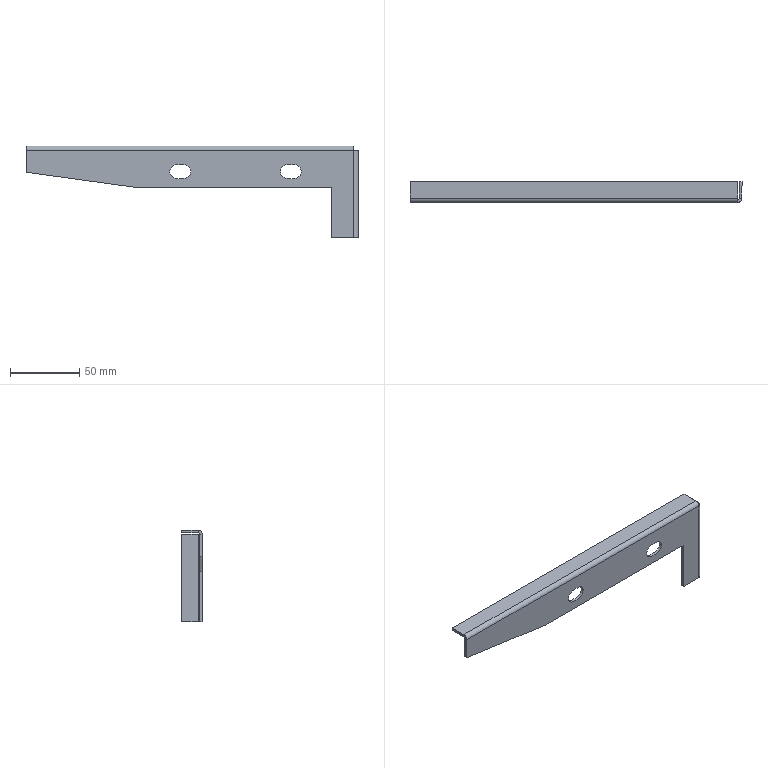Part | 1 solid | 33 faces | box 240 x 15 x 66.5 mm | volume 21672 mm3 | plane 25 | cylinder 8 | commonest cylinder face diameters 10 x4 2 x2 6 x2
STEP:
#1=CARTESIAN_POINT('',(-128.,-2.,43.));
#2=VERTEX_POINT('',#1);
#3=CARTESIAN_POINT('',(-123.,-2.,43.));
#4=VERTEX_POINT('',#3);
#5=CARTESIAN_POINT('',(-128.,-2.,43.));
#6=DIRECTION('',(1.,0.,0.));
#7=VECTOR('',#6,1000.);
#8=LINE('',#5,#7);
#9=EDGE_CURVE('',#2,#4,#8,.T.);
#10=ORIENTED_EDGE('',*,*,#9,.F.);
#11=CARTESIAN_POINT('',(-128.,-2.,53.));
#12=VERTEX_POINT('',#11);
#13=CARTESIAN_POINT('',(-128.,-2.,48.));
#14=DIRECTION('',(0.,-1.,0.));
#15=DIRECTION('',(0.,0.,-1.));
#16=AXIS2_PLACEMENT_3D('',#13,#14,#15);
#17=CIRCLE('',#16,5.);
#18=EDGE_CURVE('',#12,#2,#17,.T.);
#19=ORIENTED_EDGE('',*,*,#18,.F.);
#20=CARTESIAN_POINT('',(-123.,-2.,53.));
#21=VERTEX_POINT('',#20);
#22=CARTESIAN_POINT('',(-128.,-2.,53.));
#23=DIRECTION('',(-1.,0.,0.));
#24=VECTOR('',#23,1000.);
#25=LINE('',#22,#24);
#26=EDGE_CURVE('',#21,#12,#25,.T.);
#27=ORIENTED_EDGE('',*,*,#26,.F.);
#28=CARTESIAN_POINT('',(-123.,-2.,48.));
#29=DIRECTION('',(0.,-1.,0.));
#30=DIRECTION('',(0.,0.,-1.));
#31=AXIS2_PLACEMENT_3D('',#28,#29,#30);
#32=CIRCLE('',#31,5.);
#33=EDGE_CURVE('',#4,#21,#32,.T.);
#34=ORIENTED_EDGE('',*,*,#33,.F.);
#35=EDGE_LOOP('',(#10,#19,#27,#34));
#36=FACE_BOUND('',#35,.T.);
#37=CARTESIAN_POINT('',(-48.,-2.,43.));
#38=VERTEX_POINT('',#37);
#39=CARTESIAN_POINT('',(-43.,-2.,43.));
#40=VERTEX_POINT('',#39);
#41=CARTESIAN_POINT('',(-48.,-2.,43.));
#42=DIRECTION('',(1.,0.,0.));
#43=VECTOR('',#42,1000.);
#44=LINE('',#41,#43);
#45=EDGE_CURVE('',#38,#40,#44,.T.);
#46=ORIENTED_EDGE('',*,*,#45,.F.);
#47=CARTESIAN_POINT('',(-48.,-2.,53.));
#48=VERTEX_POINT('',#47);
#49=CARTESIAN_POINT('',(-48.,-2.,48.));
#50=DIRECTION('',(0.,-1.,0.));
#51=DIRECTION('',(0.,0.,-1.));
#52=AXIS2_PLACEMENT_3D('',#49,#50,#51);
#53=CIRCLE('',#52,5.);
#54=EDGE_CURVE('',#48,#38,#53,.T.);
#55=ORIENTED_EDGE('',*,*,#54,.F.);
#56=CARTESIAN_POINT('',(-43.,-2.,53.));
#57=VERTEX_POINT('',#56);
#58=CARTESIAN_POINT('',(-48.,-2.,53.));
#59=DIRECTION('',(-1.,0.,0.));
#60=VECTOR('',#59,1000.);
#61=LINE('',#58,#60);
#62=EDGE_CURVE('',#57,#48,#61,.T.);
#63=ORIENTED_EDGE('',*,*,#62,.F.);
#64=CARTESIAN_POINT('',(-43.,-2.,48.));
#65=DIRECTION('',(0.,-1.,0.));
#66=DIRECTION('',(0.,0.,-1.));
#67=AXIS2_PLACEMENT_3D('',#64,#65,#66);
#68=CIRCLE('',#67,5.);
#69=EDGE_CURVE('',#40,#57,#68,.T.);
#70=ORIENTED_EDGE('',*,*,#69,.F.);
#71=EDGE_LOOP('',(#46,#55,#63,#70));
#72=FACE_BOUND('',#71,.T.);
#73=CARTESIAN_POINT('',(-237.,-2.,63.5));
#74=VERTEX_POINT('',#73);
#75=CARTESIAN_POINT('',(-237.,-2.,47.5));
#76=VERTEX_POINT('',#75);
#77=CARTESIAN_POINT('',(-237.,-2.,63.5));
#78=DIRECTION('',(0.,0.,-1.));
#79=VECTOR('',#78,1000.);
#80=LINE('',#77,#79);
#81=EDGE_CURVE('',#74,#76,#80,.T.);
#82=ORIENTED_EDGE('',*,*,#81,.T.);
#83=CARTESIAN_POINT('',(-157.,-2.,36.5));
#84=VERTEX_POINT('',#83);
#85=CARTESIAN_POINT('',(-237.,-2.,47.5));
#86=DIRECTION('',(-0.9907,0.,0.1362));
#87=VECTOR('',#86,1000.);
#88=LINE('',#85,#87);
#89=EDGE_CURVE('',#84,#76,#88,.T.);
#90=ORIENTED_EDGE('',*,*,#89,.F.);
#91=CARTESIAN_POINT('',(-16.,-2.,36.5));
#92=VERTEX_POINT('',#91);
#93=CARTESIAN_POINT('',(-237.,-2.,36.5));
#94=DIRECTION('',(-1.,0.,0.));
#95=VECTOR('',#94,1000.);
#96=LINE('',#93,#95);
#97=EDGE_CURVE('',#92,#84,#96,.T.);
#98=ORIENTED_EDGE('',*,*,#97,.F.);
#99=CARTESIAN_POINT('',(-16.,-2.,0.));
#100=VERTEX_POINT('',#99);
#101=CARTESIAN_POINT('',(-16.,-2.,0.));
#102=DIRECTION('',(0.,0.,1.));
#103=VECTOR('',#102,1000.);
#104=LINE('',#101,#103);
#105=EDGE_CURVE('',#100,#92,#104,.T.);
#106=ORIENTED_EDGE('',*,*,#105,.F.);
#107=CARTESIAN_POINT('',(0.,-2.,0.));
#108=VERTEX_POINT('',#107);
#109=CARTESIAN_POINT('',(-237.,-2.,0.));
#110=DIRECTION('',(1.,0.,0.));
#111=VECTOR('',#110,1000.);
#112=LINE('',#109,#111);
#113=EDGE_CURVE('',#100,#108,#112,.T.);
#114=ORIENTED_EDGE('',*,*,#113,.T.);
#115=CARTESIAN_POINT('',(0.,-2.,63.5));
#116=VERTEX_POINT('',#115);
#117=CARTESIAN_POINT('',(0.,-2.,63.5));
#118=DIRECTION('',(0.,0.,-1.));
#119=VECTOR('',#118,1000.);
#120=LINE('',#117,#119);
#121=EDGE_CURVE('',#116,#108,#120,.T.);
#122=ORIENTED_EDGE('',*,*,#121,.F.);
#123=CARTESIAN_POINT('',(-237.,-2.,63.5));
#124=DIRECTION('',(1.,0.,0.));
#125=VECTOR('',#124,1000.);
#126=LINE('',#123,#125);
#127=EDGE_CURVE('',#74,#116,#126,.T.);
#128=ORIENTED_EDGE('',*,*,#127,.F.);
#129=EDGE_LOOP('',(#82,#90,#98,#106,#114,#122,#128));
#130=FACE_OUTER_BOUND('',#129,.T.);
#131=CARTESIAN_POINT('',(-237.,-2.,63.5));
#132=DIRECTION('',(0.,1.,0.));
#133=DIRECTION('',(0.,0.,1.));
#134=AXIS2_PLACEMENT_3D('',#131,#132,#133);
#135=PLANE('',#134);
#136=ADVANCED_FACE('',(#36,#72,#130),#135,.F.);
#137=CARTESIAN_POINT('',(-237.,0.,47.5));
#138=VERTEX_POINT('',#137);
#139=CARTESIAN_POINT('',(-157.,0.,36.5));
#140=VERTEX_POINT('',#139);
#141=CARTESIAN_POINT('',(-239.159,0.,47.797));
#142=DIRECTION('',(0.9907,0.,-0.1362));
#143=VECTOR('',#142,1000.);
#144=LINE('',#141,#143);
#145=EDGE_CURVE('',#138,#140,#144,.T.);
#146=ORIENTED_EDGE('',*,*,#145,.F.);
#147=CARTESIAN_POINT('',(-237.,0.,63.5));
#148=VERTEX_POINT('',#147);
#149=CARTESIAN_POINT('',(-237.,0.,63.5));
#150=DIRECTION('',(0.,0.,-1.));
#151=VECTOR('',#150,1000.);
#152=LINE('',#149,#151);
#153=EDGE_CURVE('',#148,#138,#152,.T.);
#154=ORIENTED_EDGE('',*,*,#153,.F.);
#155=CARTESIAN_POINT('',(0.,0.,63.5));
#156=VERTEX_POINT('',#155);
#157=CARTESIAN_POINT('',(-237.,0.,63.5));
#158=DIRECTION('',(1.,0.,0.));
#159=VECTOR('',#158,1000.);
#160=LINE('',#157,#159);
#161=EDGE_CURVE('',#148,#156,#160,.T.);
#162=ORIENTED_EDGE('',*,*,#161,.T.);
#163=CARTESIAN_POINT('',(0.,0.,0.));
#164=VERTEX_POINT('',#163);
#165=CARTESIAN_POINT('',(0.,0.,63.5));
#166=DIRECTION('',(0.,0.,-1.));
#167=VECTOR('',#166,1000.);
#168=LINE('',#165,#167);
#169=EDGE_CURVE('',#156,#164,#168,.T.);
#170=ORIENTED_EDGE('',*,*,#169,.T.);
#171=CARTESIAN_POINT('',(-16.,0.,0.));
#172=VERTEX_POINT('',#171);
#173=CARTESIAN_POINT('',(-237.,0.,0.));
#174=DIRECTION('',(1.,0.,0.));
#175=VECTOR('',#174,1000.);
#176=LINE('',#173,#175);
#177=EDGE_CURVE('',#172,#164,#176,.T.);
#178=ORIENTED_EDGE('',*,*,#177,.F.);
#179=CARTESIAN_POINT('',(-16.,0.,36.5));
#180=VERTEX_POINT('',#179);
#181=CARTESIAN_POINT('',(-16.,0.,63.5));
#182=DIRECTION('',(0.,0.,-1.));
#183=VECTOR('',#182,1000.);
#184=LINE('',#181,#183);
#185=EDGE_CURVE('',#180,#172,#184,.T.);
#186=ORIENTED_EDGE('',*,*,#185,.F.);
#187=CARTESIAN_POINT('',(-237.,0.,36.5));
#188=DIRECTION('',(1.,0.,0.));
#189=VECTOR('',#188,1000.);
#190=LINE('',#187,#189);
#191=EDGE_CURVE('',#140,#180,#190,.T.);
#192=ORIENTED_EDGE('',*,*,#191,.F.);
#193=EDGE_LOOP('',(#146,#154,#162,#170,#178,#186,#192));
#194=FACE_OUTER_BOUND('',#193,.T.);
#195=CARTESIAN_POINT('',(-128.,0.,43.));
#196=VERTEX_POINT('',#195);
#197=CARTESIAN_POINT('',(-128.,0.,53.));
#198=VERTEX_POINT('',#197);
#199=CARTESIAN_POINT('',(-128.,0.,48.));
#200=DIRECTION('',(0.,1.,0.));
#201=DIRECTION('',(0.,0.,1.));
#202=AXIS2_PLACEMENT_3D('',#199,#200,#201);
#203=CIRCLE('',#202,5.);
#204=EDGE_CURVE('',#196,#198,#203,.T.);
#205=ORIENTED_EDGE('',*,*,#204,.F.);
#206=CARTESIAN_POINT('',(-123.,0.,43.));
#207=VERTEX_POINT('',#206);
#208=CARTESIAN_POINT('',(-237.,0.,43.));
#209=DIRECTION('',(-1.,0.,0.));
#210=VECTOR('',#209,1000.);
#211=LINE('',#208,#210);
#212=EDGE_CURVE('',#207,#196,#211,.T.);
#213=ORIENTED_EDGE('',*,*,#212,.F.);
#214=CARTESIAN_POINT('',(-123.,0.,53.));
#215=VERTEX_POINT('',#214);
#216=CARTESIAN_POINT('',(-123.,0.,48.));
#217=DIRECTION('',(0.,1.,0.));
#218=DIRECTION('',(0.,0.,1.));
#219=AXIS2_PLACEMENT_3D('',#216,#217,#218);
#220=CIRCLE('',#219,5.);
#221=EDGE_CURVE('',#215,#207,#220,.T.);
#222=ORIENTED_EDGE('',*,*,#221,.F.);
#223=CARTESIAN_POINT('',(-237.,0.,53.));
#224=DIRECTION('',(1.,0.,0.));
#225=VECTOR('',#224,1000.);
#226=LINE('',#223,#225);
#227=EDGE_CURVE('',#198,#215,#226,.T.);
#228=ORIENTED_EDGE('',*,*,#227,.F.);
#229=EDGE_LOOP('',(#205,#213,#222,#228));
#230=FACE_BOUND('',#229,.T.);
#231=CARTESIAN_POINT('',(-48.,0.,43.));
#232=VERTEX_POINT('',#231);
#233=CARTESIAN_POINT('',(-48.,0.,53.));
#234=VERTEX_POINT('',#233);
#235=CARTESIAN_POINT('',(-48.,0.,48.));
#236=DIRECTION('',(0.,1.,0.));
#237=DIRECTION('',(0.,0.,1.));
#238=AXIS2_PLACEMENT_3D('',#235,#236,#237);
#239=CIRCLE('',#238,5.);
#240=EDGE_CURVE('',#232,#234,#239,.T.);
#241=ORIENTED_EDGE('',*,*,#240,.F.);
#242=CARTESIAN_POINT('',(-43.,0.,43.));
#243=VERTEX_POINT('',#242);
#244=CARTESIAN_POINT('',(-237.,0.,43.));
#245=DIRECTION('',(-1.,0.,0.));
#246=VECTOR('',#245,1000.);
#247=LINE('',#244,#246);
#248=EDGE_CURVE('',#243,#232,#247,.T.);
#249=ORIENTED_EDGE('',*,*,#248,.F.);
#250=CARTESIAN_POINT('',(-43.,0.,53.));
#251=VERTEX_POINT('',#250);
#252=CARTESIAN_POINT('',(-43.,0.,48.));
#253=DIRECTION('',(0.,1.,0.));
#254=DIRECTION('',(0.,0.,1.));
#255=AXIS2_PLACEMENT_3D('',#252,#253,#254);
#256=CIRCLE('',#255,5.);
#257=EDGE_CURVE('',#251,#243,#256,.T.);
#258=ORIENTED_EDGE('',*,*,#257,.F.);
#259=CARTESIAN_POINT('',(-237.,0.,53.));
#260=DIRECTION('',(1.,0.,0.));
#261=VECTOR('',#260,1000.);
#262=LINE('',#259,#261);
#263=EDGE_CURVE('',#234,#251,#262,.T.);
#264=ORIENTED_EDGE('',*,*,#263,.F.);
#265=EDGE_LOOP('',(#241,#249,#258,#264));
#266=FACE_BOUND('',#265,.T.);
#267=CARTESIAN_POINT('',(-237.,0.,63.5));
#268=DIRECTION('',(0.,1.,0.));
#269=DIRECTION('',(0.,0.,1.));
#270=AXIS2_PLACEMENT_3D('',#267,#268,#269);
#271=PLANE('',#270);
#272=ADVANCED_FACE('',(#194,#230,#266),#271,.T.);
#273=CARTESIAN_POINT('',(-237.,8.,47.5));
#274=DIRECTION('',(0.,-1.,0.));
#275=VECTOR('',#274,1000.);
#276=LINE('',#273,#275);
#277=EDGE_CURVE('',#138,#76,#276,.T.);
#278=ORIENTED_EDGE('',*,*,#277,.T.);
#279=ORIENTED_EDGE('',*,*,#81,.F.);
#280=CARTESIAN_POINT('',(-237.,-2.,63.5));
#281=DIRECTION('',(0.,1.,0.));
#282=VECTOR('',#281,1000.);
#283=LINE('',#280,#282);
#284=EDGE_CURVE('',#74,#148,#283,.T.);
#285=ORIENTED_EDGE('',*,*,#284,.T.);
#286=ORIENTED_EDGE('',*,*,#153,.T.);
#287=EDGE_LOOP('',(#278,#279,#285,#286));
#288=FACE_OUTER_BOUND('',#287,.T.);
#289=CARTESIAN_POINT('',(-237.,-2.,63.5));
#290=DIRECTION('',(-1.,0.,0.));
#291=DIRECTION('',(0.,0.,1.));
#292=AXIS2_PLACEMENT_3D('',#289,#290,#291);
#293=PLANE('',#292);
#294=ADVANCED_FACE('',(#288),#293,.T.);
#295=CARTESIAN_POINT('',(-16.,0.,0.));
#296=DIRECTION('',(0.,-1.,0.));
#297=VECTOR('',#296,1000.);
#298=LINE('',#295,#297);
#299=EDGE_CURVE('',#172,#100,#298,.T.);
#300=ORIENTED_EDGE('',*,*,#299,.F.);
#301=ORIENTED_EDGE('',*,*,#177,.T.);
#302=CARTESIAN_POINT('',(0.,0.,0.));
#303=DIRECTION('',(0.,-1.,0.));
#304=VECTOR('',#303,1000.);
#305=LINE('',#302,#304);
#306=EDGE_CURVE('',#164,#108,#305,.T.);
#307=ORIENTED_EDGE('',*,*,#306,.T.);
#308=ORIENTED_EDGE('',*,*,#113,.F.);
#309=EDGE_LOOP('',(#300,#301,#307,#308));
#310=FACE_OUTER_BOUND('',#309,.T.);
#311=CARTESIAN_POINT('',(0.,0.,0.));
#312=DIRECTION('',(0.,0.,-1.));
#313=DIRECTION('',(-1.,0.,0.));
#314=AXIS2_PLACEMENT_3D('',#311,#312,#313);
#315=PLANE('',#314);
#316=ADVANCED_FACE('',(#310),#315,.T.);
#317=CARTESIAN_POINT('',(-237.,1.,64.5));
#318=VERTEX_POINT('',#317);
#319=CARTESIAN_POINT('',(-237.,1.,66.5));
#320=VERTEX_POINT('',#319);
#321=CARTESIAN_POINT('',(-237.,1.,66.5));
#322=DIRECTION('',(0.,0.,1.));
#323=VECTOR('',#322,1000.);
#324=LINE('',#321,#323);
#325=EDGE_CURVE('',#318,#320,#324,.T.);
#326=ORIENTED_EDGE('',*,*,#325,.F.);
#327=CARTESIAN_POINT('',(-237.,1.,63.5));
#328=DIRECTION('',(-1.,0.,0.));
#329=DIRECTION('',(0.,0.,-1.));
#330=AXIS2_PLACEMENT_3D('',#327,#328,#329);
#331=CIRCLE('',#330,1.);
#332=EDGE_CURVE('',#148,#318,#331,.T.);
#333=ORIENTED_EDGE('',*,*,#332,.F.);
#334=ORIENTED_EDGE('',*,*,#284,.F.);
#335=CARTESIAN_POINT('',(-237.,1.,63.5));
#336=DIRECTION('',(-1.,0.,0.));
#337=DIRECTION('',(0.,0.,-1.));
#338=AXIS2_PLACEMENT_3D('',#335,#336,#337);
#339=CIRCLE('',#338,3.);
#340=EDGE_CURVE('',#74,#320,#339,.T.);
#341=ORIENTED_EDGE('',*,*,#340,.T.);
#342=EDGE_LOOP('',(#326,#333,#334,#341));
#343=FACE_OUTER_BOUND('',#342,.T.);
#344=CARTESIAN_POINT('',(-237.,1.,63.5));
#345=DIRECTION('',(-1.,0.,0.));
#346=DIRECTION('',(0.,0.,1.));
#347=AXIS2_PLACEMENT_3D('',#344,#345,#346);
#348=PLANE('',#347);
#349=ADVANCED_FACE('',(#343),#348,.T.);
#350=CARTESIAN_POINT('',(0.,1.,64.5));
#351=VERTEX_POINT('',#350);
#352=CARTESIAN_POINT('',(0.,1.,63.5));
#353=DIRECTION('',(1.,0.,0.));
#354=DIRECTION('',(0.,0.,-1.));
#355=AXIS2_PLACEMENT_3D('',#352,#353,#354);
#356=CIRCLE('',#355,1.);
#357=EDGE_CURVE('',#351,#156,#356,.T.);
#358=ORIENTED_EDGE('',*,*,#357,.F.);
#359=CARTESIAN_POINT('',(0.,1.,66.5));
#360=VERTEX_POINT('',#359);
#361=CARTESIAN_POINT('',(0.,1.,64.5));
#362=DIRECTION('',(0.,0.,1.));
#363=VECTOR('',#362,1000.);
#364=LINE('',#361,#363);
#365=EDGE_CURVE('',#351,#360,#364,.T.);
#366=ORIENTED_EDGE('',*,*,#365,.T.);
#367=CARTESIAN_POINT('',(0.,1.,63.5));
#368=DIRECTION('',(1.,0.,0.));
#369=DIRECTION('',(0.,0.,-1.));
#370=AXIS2_PLACEMENT_3D('',#367,#368,#369);
#371=CIRCLE('',#370,3.);
#372=EDGE_CURVE('',#360,#116,#371,.T.);
#373=ORIENTED_EDGE('',*,*,#372,.T.);
#374=CARTESIAN_POINT('',(0.,0.,63.5));
#375=DIRECTION('',(0.,-1.,0.));
#376=VECTOR('',#375,1000.);
#377=LINE('',#374,#376);
#378=EDGE_CURVE('',#156,#116,#377,.T.);
#379=ORIENTED_EDGE('',*,*,#378,.F.);
#380=EDGE_LOOP('',(#358,#366,#373,#379));
#381=FACE_OUTER_BOUND('',#380,.T.);
#382=CARTESIAN_POINT('',(0.,1.,63.5));
#383=DIRECTION('',(-1.,0.,0.));
#384=DIRECTION('',(0.,0.,1.));
#385=AXIS2_PLACEMENT_3D('',#382,#383,#384);
#386=PLANE('',#385);
#387=ADVANCED_FACE('',(#381),#386,.F.);
#388=ORIENTED_EDGE('',*,*,#127,.T.);
#389=ORIENTED_EDGE('',*,*,#372,.F.);
#390=CARTESIAN_POINT('',(-237.,1.,66.5));
#391=DIRECTION('',(-1.,0.,0.));
#392=VECTOR('',#391,1000.);
#393=LINE('',#390,#392);
#394=EDGE_CURVE('',#360,#320,#393,.T.);
#395=ORIENTED_EDGE('',*,*,#394,.T.);
#396=ORIENTED_EDGE('',*,*,#340,.F.);
#397=EDGE_LOOP('',(#388,#389,#395,#396));
#398=FACE_OUTER_BOUND('',#397,.T.);
#399=CARTESIAN_POINT('',(0.,1.,63.5));
#400=DIRECTION('',(1.,0.,0.));
#401=DIRECTION('',(0.,0.,1.));
#402=AXIS2_PLACEMENT_3D('',#399,#400,#401);
#403=CYLINDRICAL_SURFACE('',#402,3.);
#404=ADVANCED_FACE('',(#398),#403,.T.);
#405=ORIENTED_EDGE('',*,*,#161,.F.);
#406=ORIENTED_EDGE('',*,*,#332,.T.);
#407=CARTESIAN_POINT('',(-237.,1.,64.5));
#408=DIRECTION('',(1.,0.,0.));
#409=VECTOR('',#408,1000.);
#410=LINE('',#407,#409);
#411=EDGE_CURVE('',#318,#351,#410,.T.);
#412=ORIENTED_EDGE('',*,*,#411,.T.);
#413=ORIENTED_EDGE('',*,*,#357,.T.);
#414=EDGE_LOOP('',(#405,#406,#412,#413));
#415=FACE_OUTER_BOUND('',#414,.T.);
#416=CARTESIAN_POINT('',(0.,1.,63.5));
#417=DIRECTION('',(1.,0.,0.));
#418=DIRECTION('',(0.,0.,1.));
#419=AXIS2_PLACEMENT_3D('',#416,#417,#418);
#420=CYLINDRICAL_SURFACE('',#419,1.);
#421=ADVANCED_FACE('',(#415),#420,.F.);
#422=ORIENTED_EDGE('',*,*,#325,.T.);
#423=CARTESIAN_POINT('',(-237.,13.,66.5));
#424=VERTEX_POINT('',#423);
#425=CARTESIAN_POINT('',(-237.,0.,66.5));
#426=DIRECTION('',(0.,-1.,0.));
#427=VECTOR('',#426,1000.);
#428=LINE('',#425,#427);
#429=EDGE_CURVE('',#424,#320,#428,.T.);
#430=ORIENTED_EDGE('',*,*,#429,.F.);
#431=CARTESIAN_POINT('',(-237.,13.,64.5));
#432=VERTEX_POINT('',#431);
#433=CARTESIAN_POINT('',(-237.,13.,66.5));
#434=DIRECTION('',(0.,0.,-1.));
#435=VECTOR('',#434,1000.);
#436=LINE('',#433,#435);
#437=EDGE_CURVE('',#424,#432,#436,.T.);
#438=ORIENTED_EDGE('',*,*,#437,.T.);
#439=CARTESIAN_POINT('',(-237.,0.,64.5));
#440=DIRECTION('',(0.,-1.,0.));
#441=VECTOR('',#440,1000.);
#442=LINE('',#439,#441);
#443=EDGE_CURVE('',#432,#318,#442,.T.);
#444=ORIENTED_EDGE('',*,*,#443,.T.);
#445=EDGE_LOOP('',(#422,#430,#438,#444));
#446=FACE_OUTER_BOUND('',#445,.T.);
#447=CARTESIAN_POINT('',(-237.,0.,66.5));
#448=DIRECTION('',(1.,0.,0.));
#449=DIRECTION('',(0.,0.,-1.));
#450=AXIS2_PLACEMENT_3D('',#447,#448,#449);
#451=PLANE('',#450);
#452=ADVANCED_FACE('',(#446),#451,.F.);
#453=ORIENTED_EDGE('',*,*,#365,.F.);
#454=CARTESIAN_POINT('',(0.,13.,64.5));
#455=VERTEX_POINT('',#454);
#456=CARTESIAN_POINT('',(0.,13.,64.5));
#457=DIRECTION('',(0.,1.,0.));
#458=VECTOR('',#457,1000.);
#459=LINE('',#456,#458);
#460=EDGE_CURVE('',#351,#455,#459,.T.);
#461=ORIENTED_EDGE('',*,*,#460,.T.);
#462=CARTESIAN_POINT('',(0.,13.,66.5));
#463=VERTEX_POINT('',#462);
#464=CARTESIAN_POINT('',(0.,13.,66.5));
#465=DIRECTION('',(0.,0.,-1.));
#466=VECTOR('',#465,1000.);
#467=LINE('',#464,#466);
#468=EDGE_CURVE('',#463,#455,#467,.T.);
#469=ORIENTED_EDGE('',*,*,#468,.F.);
#470=CARTESIAN_POINT('',(0.,0.,66.5));
#471=DIRECTION('',(0.,1.,0.));
#472=VECTOR('',#471,1000.);
#473=LINE('',#470,#472);
#474=EDGE_CURVE('',#360,#463,#473,.T.);
#475=ORIENTED_EDGE('',*,*,#474,.F.);
#476=EDGE_LOOP('',(#453,#461,#469,#475));
#477=FACE_OUTER_BOUND('',#476,.T.);
#478=CARTESIAN_POINT('',(0.,13.,66.5));
#479=DIRECTION('',(-1.,0.,0.));
#480=DIRECTION('',(0.,0.,1.));
#481=AXIS2_PLACEMENT_3D('',#478,#479,#480);
#482=PLANE('',#481);
#483=ADVANCED_FACE('',(#477),#482,.F.);
#484=ORIENTED_EDGE('',*,*,#394,.F.);
#485=ORIENTED_EDGE('',*,*,#474,.T.);
#486=CARTESIAN_POINT('',(0.,13.,66.5));
#487=DIRECTION('',(-1.,0.,0.));
#488=VECTOR('',#487,1000.);
#489=LINE('',#486,#488);
#490=EDGE_CURVE('',#463,#424,#489,.T.);
#491=ORIENTED_EDGE('',*,*,#490,.T.);
#492=ORIENTED_EDGE('',*,*,#429,.T.);
#493=EDGE_LOOP('',(#484,#485,#491,#492));
#494=FACE_OUTER_BOUND('',#493,.T.);
#495=CARTESIAN_POINT('',(0.,0.,66.5));
#496=DIRECTION('',(0.,0.,-1.));
#497=DIRECTION('',(-1.,0.,0.));
#498=AXIS2_PLACEMENT_3D('',#495,#496,#497);
#499=PLANE('',#498);
#500=ADVANCED_FACE('',(#494),#499,.F.);
#501=ORIENTED_EDGE('',*,*,#460,.F.);
#502=ORIENTED_EDGE('',*,*,#411,.F.);
#503=ORIENTED_EDGE('',*,*,#443,.F.);
#504=CARTESIAN_POINT('',(-237.,13.,64.5));
#505=DIRECTION('',(-1.,0.,0.));
#506=VECTOR('',#505,1000.);
#507=LINE('',#504,#506);
#508=EDGE_CURVE('',#455,#432,#507,.T.);
#509=ORIENTED_EDGE('',*,*,#508,.F.);
#510=EDGE_LOOP('',(#501,#502,#503,#509));
#511=FACE_OUTER_BOUND('',#510,.T.);
#512=CARTESIAN_POINT('',(0.,0.,64.5));
#513=DIRECTION('',(0.,0.,-1.));
#514=DIRECTION('',(-1.,0.,0.));
#515=AXIS2_PLACEMENT_3D('',#512,#513,#514);
#516=PLANE('',#515);
#517=ADVANCED_FACE('',(#511),#516,.T.);
#518=ORIENTED_EDGE('',*,*,#508,.T.);
#519=ORIENTED_EDGE('',*,*,#437,.F.);
#520=ORIENTED_EDGE('',*,*,#490,.F.);
#521=ORIENTED_EDGE('',*,*,#468,.T.);
#522=EDGE_LOOP('',(#518,#519,#520,#521));
#523=FACE_OUTER_BOUND('',#522,.T.);
#524=CARTESIAN_POINT('',(-237.,13.,66.5));
#525=DIRECTION('',(0.,-1.,0.));
#526=DIRECTION('',(0.,0.,-1.));
#527=AXIS2_PLACEMENT_3D('',#524,#525,#526);
#528=PLANE('',#527);
#529=ADVANCED_FACE('',(#523),#528,.F.);
#530=CARTESIAN_POINT('',(1.,1.,63.5));
#531=VERTEX_POINT('',#530);
#532=CARTESIAN_POINT('',(3.,1.,63.5));
#533=VERTEX_POINT('',#532);
#534=CARTESIAN_POINT('',(3.,1.,63.5));
#535=DIRECTION('',(1.,0.,0.));
#536=VECTOR('',#535,1000.);
#537=LINE('',#534,#536);
#538=EDGE_CURVE('',#531,#533,#537,.T.);
#539=ORIENTED_EDGE('',*,*,#538,.F.);
#540=CARTESIAN_POINT('',(0.,1.,63.5));
#541=DIRECTION('',(0.,0.,1.));
#542=DIRECTION('',(-1.,0.,0.));
#543=AXIS2_PLACEMENT_3D('',#540,#541,#542);
#544=CIRCLE('',#543,1.);
#545=EDGE_CURVE('',#156,#531,#544,.T.);
#546=ORIENTED_EDGE('',*,*,#545,.F.);
#547=ORIENTED_EDGE('',*,*,#378,.T.);
#548=CARTESIAN_POINT('',(0.,1.,63.5));
#549=DIRECTION('',(0.,0.,1.));
#550=DIRECTION('',(-1.,0.,0.));
#551=AXIS2_PLACEMENT_3D('',#548,#549,#550);
#552=CIRCLE('',#551,3.);
#553=EDGE_CURVE('',#116,#533,#552,.T.);
#554=ORIENTED_EDGE('',*,*,#553,.T.);
#555=EDGE_LOOP('',(#539,#546,#547,#554));
#556=FACE_OUTER_BOUND('',#555,.T.);
#557=CARTESIAN_POINT('',(0.,1.,63.5));
#558=DIRECTION('',(0.,0.,1.));
#559=DIRECTION('',(1.,0.,0.));
#560=AXIS2_PLACEMENT_3D('',#557,#558,#559);
#561=PLANE('',#560);
#562=ADVANCED_FACE('',(#556),#561,.T.);
#563=CARTESIAN_POINT('',(1.,1.,0.));
#564=VERTEX_POINT('',#563);
#565=CARTESIAN_POINT('',(0.,1.,0.));
#566=DIRECTION('',(0.,0.,-1.));
#567=DIRECTION('',(-1.,0.,0.));
#568=AXIS2_PLACEMENT_3D('',#565,#566,#567);
#569=CIRCLE('',#568,1.);
#570=EDGE_CURVE('',#564,#164,#569,.T.);
#571=ORIENTED_EDGE('',*,*,#570,.F.);
#572=CARTESIAN_POINT('',(3.,1.,0.));
#573=VERTEX_POINT('',#572);
#574=CARTESIAN_POINT('',(1.,1.,0.));
#575=DIRECTION('',(1.,0.,0.));
#576=VECTOR('',#575,1000.);
#577=LINE('',#574,#576);
#578=EDGE_CURVE('',#564,#573,#577,.T.);
#579=ORIENTED_EDGE('',*,*,#578,.T.);
#580=CARTESIAN_POINT('',(0.,1.,0.));
#581=DIRECTION('',(0.,0.,-1.));
#582=DIRECTION('',(-1.,0.,0.));
#583=AXIS2_PLACEMENT_3D('',#580,#581,#582);
#584=CIRCLE('',#583,3.);
#585=EDGE_CURVE('',#573,#108,#584,.T.);
#586=ORIENTED_EDGE('',*,*,#585,.T.);
#587=ORIENTED_EDGE('',*,*,#306,.F.);
#588=EDGE_LOOP('',(#571,#579,#586,#587));
#589=FACE_OUTER_BOUND('',#588,.T.);
#590=CARTESIAN_POINT('',(0.,1.,0.));
#591=DIRECTION('',(0.,0.,1.));
#592=DIRECTION('',(1.,0.,0.));
#593=AXIS2_PLACEMENT_3D('',#590,#591,#592);
#594=PLANE('',#593);
#595=ADVANCED_FACE('',(#589),#594,.F.);
#596=ORIENTED_EDGE('',*,*,#121,.T.);
#597=ORIENTED_EDGE('',*,*,#585,.F.);
#598=CARTESIAN_POINT('',(3.,1.,63.5));
#599=DIRECTION('',(0.,0.,1.));
#600=VECTOR('',#599,1000.);
#601=LINE('',#598,#600);
#602=EDGE_CURVE('',#573,#533,#601,.T.);
#603=ORIENTED_EDGE('',*,*,#602,.T.);
#604=ORIENTED_EDGE('',*,*,#553,.F.);
#605=EDGE_LOOP('',(#596,#597,#603,#604));
#606=FACE_OUTER_BOUND('',#605,.T.);
#607=CARTESIAN_POINT('',(0.,1.,0.));
#608=DIRECTION('',(0.,0.,-1.));
#609=DIRECTION('',(1.,0.,0.));
#610=AXIS2_PLACEMENT_3D('',#607,#608,#609);
#611=CYLINDRICAL_SURFACE('',#610,3.);
#612=ADVANCED_FACE('',(#606),#611,.T.);
#613=ORIENTED_EDGE('',*,*,#169,.F.);
#614=ORIENTED_EDGE('',*,*,#545,.T.);
#615=CARTESIAN_POINT('',(1.,1.,63.5));
#616=DIRECTION('',(0.,0.,-1.));
#617=VECTOR('',#616,1000.);
#618=LINE('',#615,#617);
#619=EDGE_CURVE('',#531,#564,#618,.T.);
#620=ORIENTED_EDGE('',*,*,#619,.T.);
#621=ORIENTED_EDGE('',*,*,#570,.T.);
#622=EDGE_LOOP('',(#613,#614,#620,#621));
#623=FACE_OUTER_BOUND('',#622,.T.);
#624=CARTESIAN_POINT('',(0.,1.,0.));
#625=DIRECTION('',(0.,0.,-1.));
#626=DIRECTION('',(1.,0.,0.));
#627=AXIS2_PLACEMENT_3D('',#624,#625,#626);
#628=CYLINDRICAL_SURFACE('',#627,1.);
#629=ADVANCED_FACE('',(#623),#628,.F.);
#630=ORIENTED_EDGE('',*,*,#538,.T.);
#631=CARTESIAN_POINT('',(3.,13.,63.5));
#632=VERTEX_POINT('',#631);
#633=CARTESIAN_POINT('',(3.,0.,63.5));
#634=DIRECTION('',(0.,-1.,0.));
#635=VECTOR('',#634,1000.);
#636=LINE('',#633,#635);
#637=EDGE_CURVE('',#632,#533,#636,.T.);
#638=ORIENTED_EDGE('',*,*,#637,.F.);
#639=CARTESIAN_POINT('',(1.,13.,63.5));
#640=VERTEX_POINT('',#639);
#641=CARTESIAN_POINT('',(3.,13.,63.5));
#642=DIRECTION('',(-1.,0.,0.));
#643=VECTOR('',#642,1000.);
#644=LINE('',#641,#643);
#645=EDGE_CURVE('',#632,#640,#644,.T.);
#646=ORIENTED_EDGE('',*,*,#645,.T.);
#647=CARTESIAN_POINT('',(1.,0.,63.5));
#648=DIRECTION('',(0.,-1.,0.));
#649=VECTOR('',#648,1000.);
#650=LINE('',#647,#649);
#651=EDGE_CURVE('',#640,#531,#650,.T.);
#652=ORIENTED_EDGE('',*,*,#651,.T.);
#653=EDGE_LOOP('',(#630,#638,#646,#652));
#654=FACE_OUTER_BOUND('',#653,.T.);
#655=CARTESIAN_POINT('',(3.,0.,63.5));
#656=DIRECTION('',(0.,0.,-1.));
#657=DIRECTION('',(-1.,0.,0.));
#658=AXIS2_PLACEMENT_3D('',#655,#656,#657);
#659=PLANE('',#658);
#660=ADVANCED_FACE('',(#654),#659,.F.);
#661=ORIENTED_EDGE('',*,*,#578,.F.);
#662=CARTESIAN_POINT('',(1.,13.,0.));
#663=VERTEX_POINT('',#662);
#664=CARTESIAN_POINT('',(1.,13.,0.));
#665=DIRECTION('',(0.,1.,0.));
#666=VECTOR('',#665,1000.);
#667=LINE('',#664,#666);
#668=EDGE_CURVE('',#564,#663,#667,.T.);
#669=ORIENTED_EDGE('',*,*,#668,.T.);
#670=CARTESIAN_POINT('',(3.,13.,0.));
#671=VERTEX_POINT('',#670);
#672=CARTESIAN_POINT('',(3.,13.,0.));
#673=DIRECTION('',(-1.,0.,0.));
#674=VECTOR('',#673,1000.);
#675=LINE('',#672,#674);
#676=EDGE_CURVE('',#671,#663,#675,.T.);
#677=ORIENTED_EDGE('',*,*,#676,.F.);
#678=CARTESIAN_POINT('',(3.,0.,0.));
#679=DIRECTION('',(0.,1.,0.));
#680=VECTOR('',#679,1000.);
#681=LINE('',#678,#680);
#682=EDGE_CURVE('',#573,#671,#681,.T.);
#683=ORIENTED_EDGE('',*,*,#682,.F.);
#684=EDGE_LOOP('',(#661,#669,#677,#683));
#685=FACE_OUTER_BOUND('',#684,.T.);
#686=CARTESIAN_POINT('',(3.,13.,0.));
#687=DIRECTION('',(0.,0.,1.));
#688=DIRECTION('',(1.,0.,0.));
#689=AXIS2_PLACEMENT_3D('',#686,#687,#688);
#690=PLANE('',#689);
#691=ADVANCED_FACE('',(#685),#690,.F.);
#692=ORIENTED_EDGE('',*,*,#602,.F.);
#693=ORIENTED_EDGE('',*,*,#682,.T.);
#694=CARTESIAN_POINT('',(3.,13.,0.));
#695=DIRECTION('',(0.,0.,1.));
#696=VECTOR('',#695,1000.);
#697=LINE('',#694,#696);
#698=EDGE_CURVE('',#671,#632,#697,.T.);
#699=ORIENTED_EDGE('',*,*,#698,.T.);
#700=ORIENTED_EDGE('',*,*,#637,.T.);
#701=EDGE_LOOP('',(#692,#693,#699,#700));
#702=FACE_OUTER_BOUND('',#701,.T.);
#703=CARTESIAN_POINT('',(3.,0.,0.));
#704=DIRECTION('',(-1.,0.,0.));
#705=DIRECTION('',(0.,-1.,0.));
#706=AXIS2_PLACEMENT_3D('',#703,#704,#705);
#707=PLANE('',#706);
#708=ADVANCED_FACE('',(#702),#707,.F.);
#709=ORIENTED_EDGE('',*,*,#668,.F.);
#710=ORIENTED_EDGE('',*,*,#619,.F.);
#711=ORIENTED_EDGE('',*,*,#651,.F.);
#712=CARTESIAN_POINT('',(1.,13.,63.5));
#713=DIRECTION('',(0.,0.,1.));
#714=VECTOR('',#713,1000.);
#715=LINE('',#712,#714);
#716=EDGE_CURVE('',#663,#640,#715,.T.);
#717=ORIENTED_EDGE('',*,*,#716,.F.);
#718=EDGE_LOOP('',(#709,#710,#711,#717));
#719=FACE_OUTER_BOUND('',#718,.T.);
#720=CARTESIAN_POINT('',(1.,0.,0.));
#721=DIRECTION('',(-1.,0.,0.));
#722=DIRECTION('',(0.,-1.,0.));
#723=AXIS2_PLACEMENT_3D('',#720,#721,#722);
#724=PLANE('',#723);
#725=ADVANCED_FACE('',(#719),#724,.T.);
#726=ORIENTED_EDGE('',*,*,#716,.T.);
#727=ORIENTED_EDGE('',*,*,#645,.F.);
#728=ORIENTED_EDGE('',*,*,#698,.F.);
#729=ORIENTED_EDGE('',*,*,#676,.T.);
#730=EDGE_LOOP('',(#726,#727,#728,#729));
#731=FACE_OUTER_BOUND('',#730,.T.);
#732=CARTESIAN_POINT('',(3.,13.,63.5));
#733=DIRECTION('',(0.,-1.,0.));
#734=DIRECTION('',(1.,0.,0.));
#735=AXIS2_PLACEMENT_3D('',#732,#733,#734);
#736=PLANE('',#735);
#737=ADVANCED_FACE('',(#731),#736,.F.);
#738=ORIENTED_EDGE('',*,*,#97,.T.);
#739=CARTESIAN_POINT('',(-157.,8.,36.5));
#740=DIRECTION('',(0.,1.,0.));
#741=VECTOR('',#740,1000.);
#742=LINE('',#739,#741);
#743=EDGE_CURVE('',#84,#140,#742,.T.);
#744=ORIENTED_EDGE('',*,*,#743,.T.);
#745=ORIENTED_EDGE('',*,*,#191,.T.);
#746=CARTESIAN_POINT('',(-16.,8.,36.5));
#747=DIRECTION('',(0.,-1.,0.));
#748=VECTOR('',#747,1000.);
#749=LINE('',#746,#748);
#750=EDGE_CURVE('',#180,#92,#749,.T.);
#751=ORIENTED_EDGE('',*,*,#750,.T.);
#752=EDGE_LOOP('',(#738,#744,#745,#751));
#753=FACE_OUTER_BOUND('',#752,.T.);
#754=CARTESIAN_POINT('',(-237.,8.,36.5));
#755=DIRECTION('',(0.,0.,1.));
#756=DIRECTION('',(1.,0.,0.));
#757=AXIS2_PLACEMENT_3D('',#754,#755,#756);
#758=PLANE('',#757);
#759=ADVANCED_FACE('',(#753),#758,.F.);
#760=ORIENTED_EDGE('',*,*,#185,.T.);
#761=ORIENTED_EDGE('',*,*,#299,.T.);
#762=ORIENTED_EDGE('',*,*,#105,.T.);
#763=ORIENTED_EDGE('',*,*,#750,.F.);
#764=EDGE_LOOP('',(#760,#761,#762,#763));
#765=FACE_OUTER_BOUND('',#764,.T.);
#766=CARTESIAN_POINT('',(-16.,8.,0.));
#767=DIRECTION('',(1.,0.,0.));
#768=DIRECTION('',(0.,0.,-1.));
#769=AXIS2_PLACEMENT_3D('',#766,#767,#768);
#770=PLANE('',#769);
#771=ADVANCED_FACE('',(#765),#770,.F.);
#772=ORIENTED_EDGE('',*,*,#240,.T.);
#773=CARTESIAN_POINT('',(-48.,8.,53.));
#774=DIRECTION('',(0.,-1.,0.));
#775=VECTOR('',#774,1000.);
#776=LINE('',#773,#775);
#777=EDGE_CURVE('',#234,#48,#776,.T.);
#778=ORIENTED_EDGE('',*,*,#777,.T.);
#779=ORIENTED_EDGE('',*,*,#54,.T.);
#780=CARTESIAN_POINT('',(-48.,8.,43.));
#781=DIRECTION('',(0.,-1.,0.));
#782=VECTOR('',#781,1000.);
#783=LINE('',#780,#782);
#784=EDGE_CURVE('',#232,#38,#783,.T.);
#785=ORIENTED_EDGE('',*,*,#784,.F.);
#786=EDGE_LOOP('',(#772,#778,#779,#785));
#787=FACE_OUTER_BOUND('',#786,.T.);
#788=CARTESIAN_POINT('',(-48.,8.,48.));
#789=DIRECTION('',(0.,-1.,0.));
#790=DIRECTION('',(0.,0.,-1.));
#791=AXIS2_PLACEMENT_3D('',#788,#789,#790);
#792=CYLINDRICAL_SURFACE('',#791,5.);
#793=ADVANCED_FACE('',(#787),#792,.F.);
#794=ORIENTED_EDGE('',*,*,#263,.T.);
#795=CARTESIAN_POINT('',(-43.,8.,53.));
#796=DIRECTION('',(0.,-1.,0.));
#797=VECTOR('',#796,1000.);
#798=LINE('',#795,#797);
#799=EDGE_CURVE('',#251,#57,#798,.T.);
#800=ORIENTED_EDGE('',*,*,#799,.T.);
#801=ORIENTED_EDGE('',*,*,#62,.T.);
#802=ORIENTED_EDGE('',*,*,#777,.F.);
#803=EDGE_LOOP('',(#794,#800,#801,#802));
#804=FACE_OUTER_BOUND('',#803,.T.);
#805=CARTESIAN_POINT('',(-48.,8.,53.));
#806=DIRECTION('',(0.,0.,1.));
#807=DIRECTION('',(1.,0.,0.));
#808=AXIS2_PLACEMENT_3D('',#805,#806,#807);
#809=PLANE('',#808);
#810=ADVANCED_FACE('',(#804),#809,.F.);
#811=ORIENTED_EDGE('',*,*,#257,.T.);
#812=CARTESIAN_POINT('',(-43.,8.,43.));
#813=DIRECTION('',(0.,-1.,0.));
#814=VECTOR('',#813,1000.);
#815=LINE('',#812,#814);
#816=EDGE_CURVE('',#243,#40,#815,.T.);
#817=ORIENTED_EDGE('',*,*,#816,.T.);
#818=ORIENTED_EDGE('',*,*,#69,.T.);
#819=ORIENTED_EDGE('',*,*,#799,.F.);
#820=EDGE_LOOP('',(#811,#817,#818,#819));
#821=FACE_OUTER_BOUND('',#820,.T.);
#822=CARTESIAN_POINT('',(-43.,8.,48.));
#823=DIRECTION('',(0.,-1.,0.));
#824=DIRECTION('',(0.,0.,-1.));
#825=AXIS2_PLACEMENT_3D('',#822,#823,#824);
#826=CYLINDRICAL_SURFACE('',#825,5.);
#827=ADVANCED_FACE('',(#821),#826,.F.);
#828=ORIENTED_EDGE('',*,*,#248,.T.);
#829=ORIENTED_EDGE('',*,*,#784,.T.);
#830=ORIENTED_EDGE('',*,*,#45,.T.);
#831=ORIENTED_EDGE('',*,*,#816,.F.);
#832=EDGE_LOOP('',(#828,#829,#830,#831));
#833=FACE_OUTER_BOUND('',#832,.T.);
#834=CARTESIAN_POINT('',(-48.,8.,43.));
#835=DIRECTION('',(0.,0.,-1.));
#836=DIRECTION('',(-1.,0.,0.));
#837=AXIS2_PLACEMENT_3D('',#834,#835,#836);
#838=PLANE('',#837);
#839=ADVANCED_FACE('',(#833),#838,.F.);
#840=ORIENTED_EDGE('',*,*,#204,.T.);
#841=CARTESIAN_POINT('',(-128.,8.,53.));
#842=DIRECTION('',(0.,-1.,0.));
#843=VECTOR('',#842,1000.);
#844=LINE('',#841,#843);
#845=EDGE_CURVE('',#198,#12,#844,.T.);
#846=ORIENTED_EDGE('',*,*,#845,.T.);
#847=ORIENTED_EDGE('',*,*,#18,.T.);
#848=CARTESIAN_POINT('',(-128.,8.,43.));
#849=DIRECTION('',(0.,-1.,0.));
#850=VECTOR('',#849,1000.);
#851=LINE('',#848,#850);
#852=EDGE_CURVE('',#196,#2,#851,.T.);
#853=ORIENTED_EDGE('',*,*,#852,.F.);
#854=EDGE_LOOP('',(#840,#846,#847,#853));
#855=FACE_OUTER_BOUND('',#854,.T.);
#856=CARTESIAN_POINT('',(-128.,8.,48.));
#857=DIRECTION('',(0.,-1.,0.));
#858=DIRECTION('',(0.,0.,-1.));
#859=AXIS2_PLACEMENT_3D('',#856,#857,#858);
#860=CYLINDRICAL_SURFACE('',#859,5.);
#861=ADVANCED_FACE('',(#855),#860,.F.);
#862=ORIENTED_EDGE('',*,*,#227,.T.);
#863=CARTESIAN_POINT('',(-123.,8.,53.));
#864=DIRECTION('',(0.,-1.,0.));
#865=VECTOR('',#864,1000.);
#866=LINE('',#863,#865);
#867=EDGE_CURVE('',#215,#21,#866,.T.);
#868=ORIENTED_EDGE('',*,*,#867,.T.);
#869=ORIENTED_EDGE('',*,*,#26,.T.);
#870=ORIENTED_EDGE('',*,*,#845,.F.);
#871=EDGE_LOOP('',(#862,#868,#869,#870));
#872=FACE_OUTER_BOUND('',#871,.T.);
#873=CARTESIAN_POINT('',(-128.,8.,53.));
#874=DIRECTION('',(0.,0.,1.));
#875=DIRECTION('',(1.,0.,0.));
#876=AXIS2_PLACEMENT_3D('',#873,#874,#875);
#877=PLANE('',#876);
#878=ADVANCED_FACE('',(#872),#877,.F.);
#879=ORIENTED_EDGE('',*,*,#221,.T.);
#880=CARTESIAN_POINT('',(-123.,8.,43.));
#881=DIRECTION('',(0.,-1.,0.));
#882=VECTOR('',#881,1000.);
#883=LINE('',#880,#882);
#884=EDGE_CURVE('',#207,#4,#883,.T.);
#885=ORIENTED_EDGE('',*,*,#884,.T.);
#886=ORIENTED_EDGE('',*,*,#33,.T.);
#887=ORIENTED_EDGE('',*,*,#867,.F.);
#888=EDGE_LOOP('',(#879,#885,#886,#887));
#889=FACE_OUTER_BOUND('',#888,.T.);
#890=CARTESIAN_POINT('',(-123.,8.,48.));
#891=DIRECTION('',(0.,-1.,0.));
#892=DIRECTION('',(0.,0.,-1.));
#893=AXIS2_PLACEMENT_3D('',#890,#891,#892);
#894=CYLINDRICAL_SURFACE('',#893,5.);
#895=ADVANCED_FACE('',(#889),#894,.F.);
#896=ORIENTED_EDGE('',*,*,#212,.T.);
#897=ORIENTED_EDGE('',*,*,#852,.T.);
#898=ORIENTED_EDGE('',*,*,#9,.T.);
#899=ORIENTED_EDGE('',*,*,#884,.F.);
#900=EDGE_LOOP('',(#896,#897,#898,#899));
#901=FACE_OUTER_BOUND('',#900,.T.);
#902=CARTESIAN_POINT('',(-128.,8.,43.));
#903=DIRECTION('',(0.,0.,-1.));
#904=DIRECTION('',(-1.,0.,0.));
#905=AXIS2_PLACEMENT_3D('',#902,#903,#904);
#906=PLANE('',#905);
#907=ADVANCED_FACE('',(#901),#906,.F.);
#908=ORIENTED_EDGE('',*,*,#145,.T.);
#909=ORIENTED_EDGE('',*,*,#743,.F.);
#910=ORIENTED_EDGE('',*,*,#89,.T.);
#911=ORIENTED_EDGE('',*,*,#277,.F.);
#912=EDGE_LOOP('',(#908,#909,#910,#911));
#913=FACE_OUTER_BOUND('',#912,.T.);
#914=CARTESIAN_POINT('',(-237.,8.,47.5));
#915=DIRECTION('',(0.1362,0.,0.9907));
#916=DIRECTION('',(0.9907,0.,-0.1362));
#917=AXIS2_PLACEMENT_3D('',#914,#915,#916);
#918=PLANE('',#917);
#919=ADVANCED_FACE('',(#913),#918,.F.);
#920=CLOSED_SHELL('',(#136,#272,#294,#316,#349,#387,#404,#421,#452,#483,#500,#517,#529,#562,#595,#612,#629,#660,#691,#708,#725,#737,#759,#771,#793,#810,#827,#839,#861,#878,#895,#907,#919));
#921=MANIFOLD_SOLID_BREP('',#920);
#922=CARTESIAN_POINT('',(0.,0.,0.));
#923=DIRECTION('',(0.,0.,1.));
#924=DIRECTION('',(1.,0.,0.));
#925=AXIS2_PLACEMENT_3D('',#922,#923,#924);
#926=(LENGTH_UNIT()NAMED_UNIT(*)SI_UNIT(.MILLI.,.METRE.));
#927=UNCERTAINTY_MEASURE_WITH_UNIT(LENGTH_MEASURE(0.00001),#926,'','');
#928=(NAMED_UNIT(*)PLANE_ANGLE_UNIT()SI_UNIT($,.RADIAN.));
#929=(NAMED_UNIT(*)SI_UNIT($,.STERADIAN.)SOLID_ANGLE_UNIT());
#930=(GEOMETRIC_REPRESENTATION_CONTEXT(3)GLOBAL_UNCERTAINTY_ASSIGNED_CONTEXT((#927))GLOBAL_UNIT_ASSIGNED_CONTEXT((#926,#928,#929))REPRESENTATION_CONTEXT('',''));
#931=ADVANCED_BREP_SHAPE_REPRESENTATION('',(#921,#925),#930);